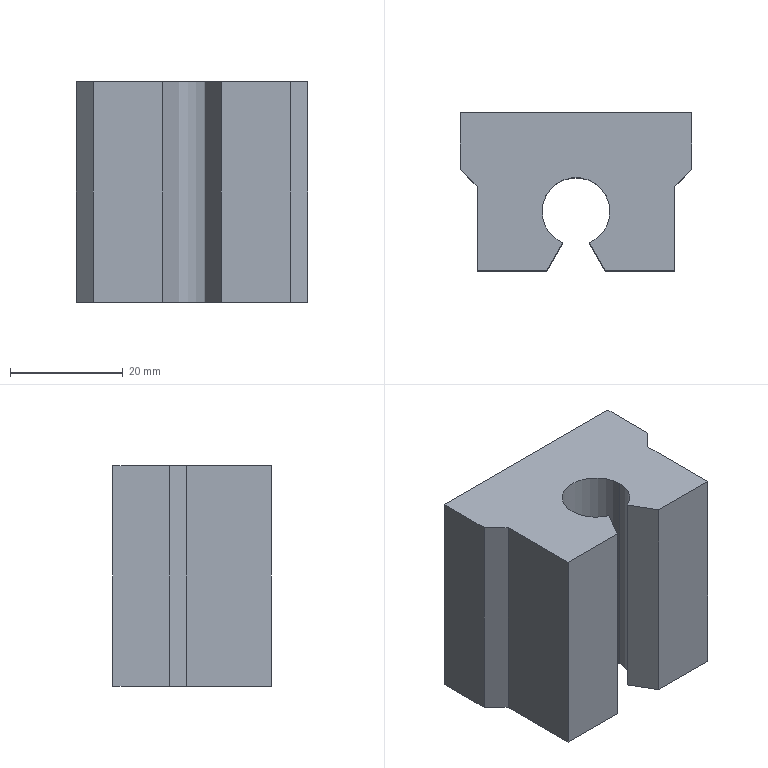Part | STEP file | SBR16S slide rail | 1 solid | 32 faces | box 41 x 28 x 39 mm | volume 34697 mm3 | plane 13 | cylinder 11 | cone 8 | commonest cylinder face diameters 3.3 x8 12 x3